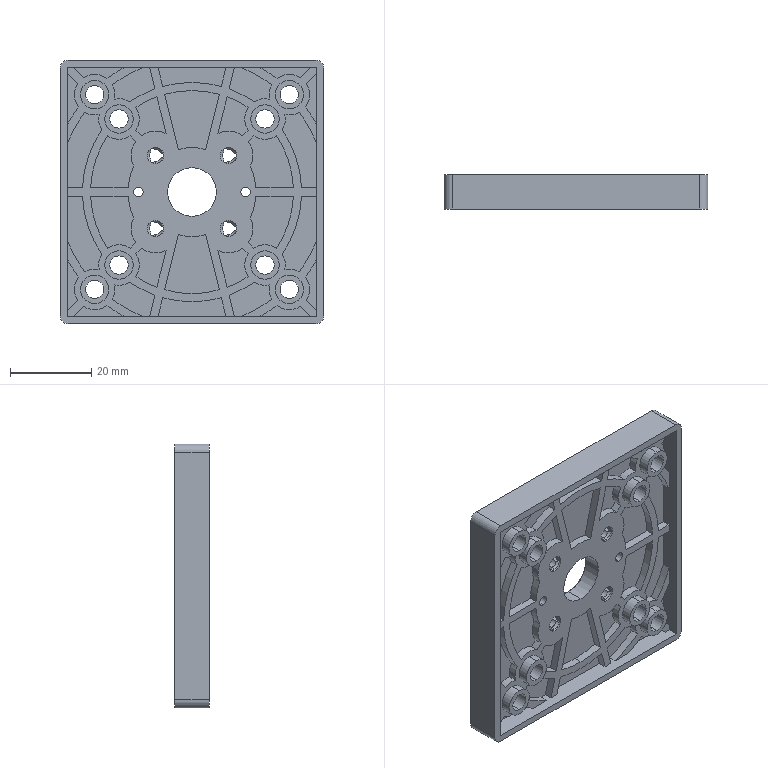Part | STEP file | PCS-P01A-2_1_2.stp | 1 solid | 426 faces | box 65 x 8.5 x 65 mm | volume 14701 mm3 | cylinder 200 | plane 142 | torus 52 | cone 32 | commonest cylinder face diameters 10 x52 2.9 x16 4.5 x16 6 x16 7 x16 4 x12